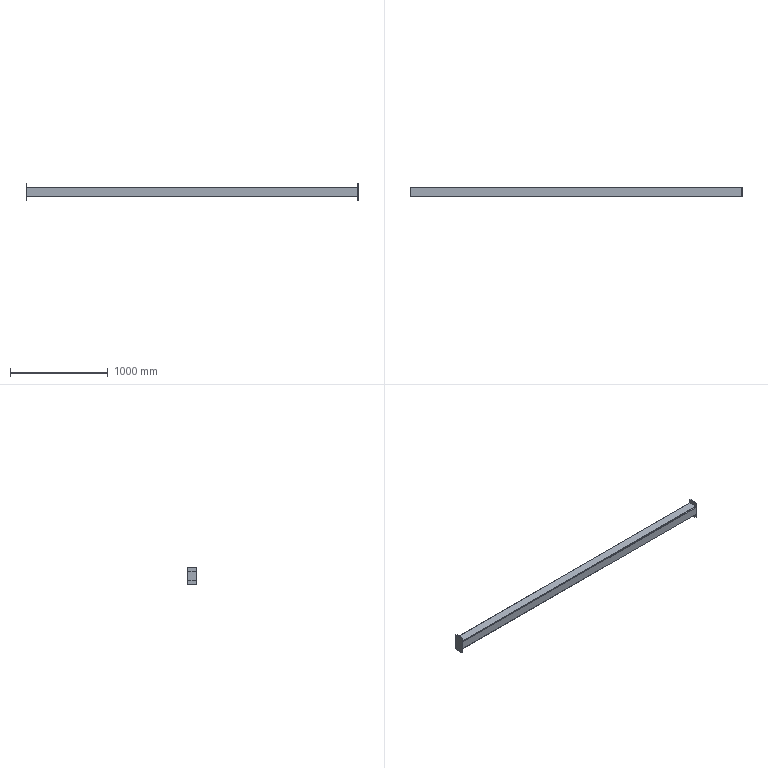Part | STEP file | Cross beam 2_Default<Machined> | 3 solids | 30 faces | box 3400 x 100 x 180 mm | volume 5412412 mm3 | plane 22 | cylinder 8 | commonest cylinder face diameters 8 x4 16 x4
STEP:
#1=CARTESIAN_POINT('',(-1690.,42.,-50.));
#2=VERTEX_POINT('',#1);
#3=CARTESIAN_POINT('',(-1690.,50.,-42.));
#4=VERTEX_POINT('',#3);
#5=CARTESIAN_POINT('',(-1690.,42.,-42.));
#6=DIRECTION('',(1.,0.,0.));
#7=DIRECTION('',(0.,0.,-1.));
#8=AXIS2_PLACEMENT_3D('',#5,#6,#7);
#9=CIRCLE('',#8,8.);
#10=EDGE_CURVE('',#2,#4,#9,.T.);
#11=ORIENTED_EDGE('',*,*,#10,.T.);
#12=CARTESIAN_POINT('',(1690.,50.,-42.));
#13=VERTEX_POINT('',#12);
#14=CARTESIAN_POINT('',(1690.,50.,-42.));
#15=DIRECTION('',(-1.,0.,0.));
#16=VECTOR('',#15,1000.);
#17=LINE('',#14,#16);
#18=EDGE_CURVE('',#13,#4,#17,.T.);
#19=ORIENTED_EDGE('',*,*,#18,.F.);
#20=CARTESIAN_POINT('',(1690.,42.,-50.));
#21=VERTEX_POINT('',#20);
#22=CARTESIAN_POINT('',(1690.,42.,-42.));
#23=DIRECTION('',(1.,0.,0.));
#24=DIRECTION('',(0.,0.,-1.));
#25=AXIS2_PLACEMENT_3D('',#22,#23,#24);
#26=CIRCLE('',#25,8.);
#27=EDGE_CURVE('',#21,#13,#26,.T.);
#28=ORIENTED_EDGE('',*,*,#27,.F.);
#29=CARTESIAN_POINT('',(1690.,42.,-50.));
#30=DIRECTION('',(-1.,0.,0.));
#31=VECTOR('',#30,1000.);
#32=LINE('',#29,#31);
#33=EDGE_CURVE('',#21,#2,#32,.T.);
#34=ORIENTED_EDGE('',*,*,#33,.T.);
#35=EDGE_LOOP('',(#11,#19,#28,#34));
#36=FACE_OUTER_BOUND('',#35,.T.);
#37=CARTESIAN_POINT('',(1690.,42.,-42.));
#38=DIRECTION('',(-1.,0.,0.));
#39=DIRECTION('',(0.,0.,1.));
#40=AXIS2_PLACEMENT_3D('',#37,#38,#39);
#41=CYLINDRICAL_SURFACE('',#40,8.);
#42=ADVANCED_FACE('',(#36),#41,.T.);
#43=CARTESIAN_POINT('',(-1690.,50.,42.));
#44=VERTEX_POINT('',#43);
#45=CARTESIAN_POINT('',(-1690.,50.,-42.));
#46=DIRECTION('',(0.,0.,1.));
#47=VECTOR('',#46,1000.);
#48=LINE('',#45,#47);
#49=EDGE_CURVE('',#4,#44,#48,.T.);
#50=ORIENTED_EDGE('',*,*,#49,.T.);
#51=CARTESIAN_POINT('',(1690.,50.,42.));
#52=VERTEX_POINT('',#51);
#53=CARTESIAN_POINT('',(1690.,50.,42.));
#54=DIRECTION('',(-1.,0.,0.));
#55=VECTOR('',#54,1000.);
#56=LINE('',#53,#55);
#57=EDGE_CURVE('',#52,#44,#56,.T.);
#58=ORIENTED_EDGE('',*,*,#57,.F.);
#59=CARTESIAN_POINT('',(1690.,50.,-42.));
#60=DIRECTION('',(0.,0.,1.));
#61=VECTOR('',#60,1000.);
#62=LINE('',#59,#61);
#63=EDGE_CURVE('',#13,#52,#62,.T.);
#64=ORIENTED_EDGE('',*,*,#63,.F.);
#65=ORIENTED_EDGE('',*,*,#18,.T.);
#66=EDGE_LOOP('',(#50,#58,#64,#65));
#67=FACE_OUTER_BOUND('',#66,.T.);
#68=CARTESIAN_POINT('',(1690.,50.,-42.));
#69=DIRECTION('',(0.,-1.,0.));
#70=DIRECTION('',(0.,0.,-1.));
#71=AXIS2_PLACEMENT_3D('',#68,#69,#70);
#72=PLANE('',#71);
#73=ADVANCED_FACE('',(#67),#72,.F.);
#74=CARTESIAN_POINT('',(-1690.,42.,50.));
#75=VERTEX_POINT('',#74);
#76=CARTESIAN_POINT('',(-1690.,42.,42.));
#77=DIRECTION('',(1.,0.,0.));
#78=DIRECTION('',(0.,0.,-1.));
#79=AXIS2_PLACEMENT_3D('',#76,#77,#78);
#80=CIRCLE('',#79,8.);
#81=EDGE_CURVE('',#44,#75,#80,.T.);
#82=ORIENTED_EDGE('',*,*,#81,.T.);
#83=CARTESIAN_POINT('',(1690.,42.,50.));
#84=VERTEX_POINT('',#83);
#85=CARTESIAN_POINT('',(1690.,42.,50.));
#86=DIRECTION('',(-1.,0.,0.));
#87=VECTOR('',#86,1000.);
#88=LINE('',#85,#87);
#89=EDGE_CURVE('',#84,#75,#88,.T.);
#90=ORIENTED_EDGE('',*,*,#89,.F.);
#91=CARTESIAN_POINT('',(1690.,42.,42.));
#92=DIRECTION('',(1.,0.,0.));
#93=DIRECTION('',(0.,0.,-1.));
#94=AXIS2_PLACEMENT_3D('',#91,#92,#93);
#95=CIRCLE('',#94,8.);
#96=EDGE_CURVE('',#52,#84,#95,.T.);
#97=ORIENTED_EDGE('',*,*,#96,.F.);
#98=ORIENTED_EDGE('',*,*,#57,.T.);
#99=EDGE_LOOP('',(#82,#90,#97,#98));
#100=FACE_OUTER_BOUND('',#99,.T.);
#101=CARTESIAN_POINT('',(1690.,42.,42.));
#102=DIRECTION('',(-1.,0.,0.));
#103=DIRECTION('',(0.,0.,1.));
#104=AXIS2_PLACEMENT_3D('',#101,#102,#103);
#105=CYLINDRICAL_SURFACE('',#104,8.);
#106=ADVANCED_FACE('',(#100),#105,.T.);
#107=CARTESIAN_POINT('',(-1690.,-42.,50.));
#108=VERTEX_POINT('',#107);
#109=CARTESIAN_POINT('',(-1690.,-42.,50.));
#110=DIRECTION('',(0.,-1.,0.));
#111=VECTOR('',#110,1000.);
#112=LINE('',#109,#111);
#113=EDGE_CURVE('',#75,#108,#112,.T.);
#114=ORIENTED_EDGE('',*,*,#113,.T.);
#115=CARTESIAN_POINT('',(1690.,-42.,50.));
#116=VERTEX_POINT('',#115);
#117=CARTESIAN_POINT('',(1690.,-42.,50.));
#118=DIRECTION('',(-1.,0.,0.));
#119=VECTOR('',#118,1000.);
#120=LINE('',#117,#119);
#121=EDGE_CURVE('',#116,#108,#120,.T.);
#122=ORIENTED_EDGE('',*,*,#121,.F.);
#123=CARTESIAN_POINT('',(1690.,-42.,50.));
#124=DIRECTION('',(0.,-1.,0.));
#125=VECTOR('',#124,1000.);
#126=LINE('',#123,#125);
#127=EDGE_CURVE('',#84,#116,#126,.T.);
#128=ORIENTED_EDGE('',*,*,#127,.F.);
#129=ORIENTED_EDGE('',*,*,#89,.T.);
#130=EDGE_LOOP('',(#114,#122,#128,#129));
#131=FACE_OUTER_BOUND('',#130,.T.);
#132=CARTESIAN_POINT('',(1690.,-42.,50.));
#133=DIRECTION('',(0.,0.,-1.));
#134=DIRECTION('',(-1.,0.,0.));
#135=AXIS2_PLACEMENT_3D('',#132,#133,#134);
#136=PLANE('',#135);
#137=ADVANCED_FACE('',(#131),#136,.F.);
#138=CARTESIAN_POINT('',(-1690.,-50.,42.));
#139=VERTEX_POINT('',#138);
#140=CARTESIAN_POINT('',(-1690.,-42.,42.));
#141=DIRECTION('',(1.,0.,0.));
#142=DIRECTION('',(0.,0.,-1.));
#143=AXIS2_PLACEMENT_3D('',#140,#141,#142);
#144=CIRCLE('',#143,8.);
#145=EDGE_CURVE('',#108,#139,#144,.T.);
#146=ORIENTED_EDGE('',*,*,#145,.T.);
#147=CARTESIAN_POINT('',(1690.,-50.,42.));
#148=VERTEX_POINT('',#147);
#149=CARTESIAN_POINT('',(1690.,-50.,42.));
#150=DIRECTION('',(-1.,0.,0.));
#151=VECTOR('',#150,1000.);
#152=LINE('',#149,#151);
#153=EDGE_CURVE('',#148,#139,#152,.T.);
#154=ORIENTED_EDGE('',*,*,#153,.F.);
#155=CARTESIAN_POINT('',(1690.,-42.,42.));
#156=DIRECTION('',(1.,0.,0.));
#157=DIRECTION('',(0.,0.,-1.));
#158=AXIS2_PLACEMENT_3D('',#155,#156,#157);
#159=CIRCLE('',#158,8.);
#160=EDGE_CURVE('',#116,#148,#159,.T.);
#161=ORIENTED_EDGE('',*,*,#160,.F.);
#162=ORIENTED_EDGE('',*,*,#121,.T.);
#163=EDGE_LOOP('',(#146,#154,#161,#162));
#164=FACE_OUTER_BOUND('',#163,.T.);
#165=CARTESIAN_POINT('',(1690.,-42.,42.));
#166=DIRECTION('',(-1.,0.,0.));
#167=DIRECTION('',(0.,0.,1.));
#168=AXIS2_PLACEMENT_3D('',#165,#166,#167);
#169=CYLINDRICAL_SURFACE('',#168,8.);
#170=ADVANCED_FACE('',(#164),#169,.T.);
#171=CARTESIAN_POINT('',(-1690.,-50.,-42.));
#172=VERTEX_POINT('',#171);
#173=CARTESIAN_POINT('',(-1690.,-50.,42.));
#174=DIRECTION('',(0.,0.,-1.));
#175=VECTOR('',#174,1000.);
#176=LINE('',#173,#175);
#177=EDGE_CURVE('',#139,#172,#176,.T.);
#178=ORIENTED_EDGE('',*,*,#177,.T.);
#179=CARTESIAN_POINT('',(1690.,-50.,-42.));
#180=VERTEX_POINT('',#179);
#181=CARTESIAN_POINT('',(1690.,-50.,-42.));
#182=DIRECTION('',(-1.,0.,0.));
#183=VECTOR('',#182,1000.);
#184=LINE('',#181,#183);
#185=EDGE_CURVE('',#180,#172,#184,.T.);
#186=ORIENTED_EDGE('',*,*,#185,.F.);
#187=CARTESIAN_POINT('',(1690.,-50.,42.));
#188=DIRECTION('',(0.,0.,-1.));
#189=VECTOR('',#188,1000.);
#190=LINE('',#187,#189);
#191=EDGE_CURVE('',#148,#180,#190,.T.);
#192=ORIENTED_EDGE('',*,*,#191,.F.);
#193=ORIENTED_EDGE('',*,*,#153,.T.);
#194=EDGE_LOOP('',(#178,#186,#192,#193));
#195=FACE_OUTER_BOUND('',#194,.T.);
#196=CARTESIAN_POINT('',(1690.,-50.,42.));
#197=DIRECTION('',(0.,1.,0.));
#198=DIRECTION('',(0.,0.,1.));
#199=AXIS2_PLACEMENT_3D('',#196,#197,#198);
#200=PLANE('',#199);
#201=ADVANCED_FACE('',(#195),#200,.F.);
#202=CARTESIAN_POINT('',(-1690.,-42.,-50.));
#203=VERTEX_POINT('',#202);
#204=CARTESIAN_POINT('',(-1690.,-42.,-42.));
#205=DIRECTION('',(1.,0.,0.));
#206=DIRECTION('',(0.,0.,-1.));
#207=AXIS2_PLACEMENT_3D('',#204,#205,#206);
#208=CIRCLE('',#207,8.);
#209=EDGE_CURVE('',#172,#203,#208,.T.);
#210=ORIENTED_EDGE('',*,*,#209,.T.);
#211=CARTESIAN_POINT('',(1690.,-42.,-50.));
#212=VERTEX_POINT('',#211);
#213=CARTESIAN_POINT('',(1690.,-42.,-50.));
#214=DIRECTION('',(-1.,0.,0.));
#215=VECTOR('',#214,1000.);
#216=LINE('',#213,#215);
#217=EDGE_CURVE('',#212,#203,#216,.T.);
#218=ORIENTED_EDGE('',*,*,#217,.F.);
#219=CARTESIAN_POINT('',(1690.,-42.,-42.));
#220=DIRECTION('',(1.,0.,0.));
#221=DIRECTION('',(0.,0.,-1.));
#222=AXIS2_PLACEMENT_3D('',#219,#220,#221);
#223=CIRCLE('',#222,8.);
#224=EDGE_CURVE('',#180,#212,#223,.T.);
#225=ORIENTED_EDGE('',*,*,#224,.F.);
#226=ORIENTED_EDGE('',*,*,#185,.T.);
#227=EDGE_LOOP('',(#210,#218,#225,#226));
#228=FACE_OUTER_BOUND('',#227,.T.);
#229=CARTESIAN_POINT('',(1690.,-42.,-42.));
#230=DIRECTION('',(-1.,0.,0.));
#231=DIRECTION('',(0.,0.,1.));
#232=AXIS2_PLACEMENT_3D('',#229,#230,#231);
#233=CYLINDRICAL_SURFACE('',#232,8.);
#234=ADVANCED_FACE('',(#228),#233,.T.);
#235=CARTESIAN_POINT('',(-1690.,46.,42.));
#236=VERTEX_POINT('',#235);
#237=CARTESIAN_POINT('',(-1690.,42.,46.));
#238=VERTEX_POINT('',#237);
#239=CARTESIAN_POINT('',(-1690.,42.,42.));
#240=DIRECTION('',(1.,0.,0.));
#241=DIRECTION('',(0.,0.,-1.));
#242=AXIS2_PLACEMENT_3D('',#239,#240,#241);
#243=CIRCLE('',#242,4.);
#244=EDGE_CURVE('',#236,#238,#243,.T.);
#245=ORIENTED_EDGE('',*,*,#244,.F.);
#246=CARTESIAN_POINT('',(1690.,46.,42.));
#247=VERTEX_POINT('',#246);
#248=CARTESIAN_POINT('',(1690.,46.,42.));
#249=DIRECTION('',(-1.,0.,0.));
#250=VECTOR('',#249,1000.);
#251=LINE('',#248,#250);
#252=EDGE_CURVE('',#247,#236,#251,.T.);
#253=ORIENTED_EDGE('',*,*,#252,.F.);
#254=CARTESIAN_POINT('',(1690.,42.,46.));
#255=VERTEX_POINT('',#254);
#256=CARTESIAN_POINT('',(1690.,42.,42.));
#257=DIRECTION('',(1.,0.,0.));
#258=DIRECTION('',(0.,0.,-1.));
#259=AXIS2_PLACEMENT_3D('',#256,#257,#258);
#260=CIRCLE('',#259,4.);
#261=EDGE_CURVE('',#247,#255,#260,.T.);
#262=ORIENTED_EDGE('',*,*,#261,.T.);
#263=CARTESIAN_POINT('',(1690.,42.,46.));
#264=DIRECTION('',(-1.,0.,0.));
#265=VECTOR('',#264,1000.);
#266=LINE('',#263,#265);
#267=EDGE_CURVE('',#255,#238,#266,.T.);
#268=ORIENTED_EDGE('',*,*,#267,.T.);
#269=EDGE_LOOP('',(#245,#253,#262,#268));
#270=FACE_OUTER_BOUND('',#269,.T.);
#271=CARTESIAN_POINT('',(1690.,42.,42.));
#272=DIRECTION('',(-1.,0.,0.));
#273=DIRECTION('',(0.,0.,1.));
#274=AXIS2_PLACEMENT_3D('',#271,#272,#273);
#275=CYLINDRICAL_SURFACE('',#274,4.);
#276=ADVANCED_FACE('',(#270),#275,.F.);
#277=CARTESIAN_POINT('',(-1690.,46.,-42.));
#278=VERTEX_POINT('',#277);
#279=CARTESIAN_POINT('',(-1690.,46.,-42.));
#280=DIRECTION('',(0.,0.,1.));
#281=VECTOR('',#280,1000.);
#282=LINE('',#279,#281);
#283=EDGE_CURVE('',#278,#236,#282,.T.);
#284=ORIENTED_EDGE('',*,*,#283,.F.);
#285=CARTESIAN_POINT('',(1690.,46.,-42.));
#286=VERTEX_POINT('',#285);
#287=CARTESIAN_POINT('',(1690.,46.,-42.));
#288=DIRECTION('',(-1.,0.,0.));
#289=VECTOR('',#288,1000.);
#290=LINE('',#287,#289);
#291=EDGE_CURVE('',#286,#278,#290,.T.);
#292=ORIENTED_EDGE('',*,*,#291,.F.);
#293=CARTESIAN_POINT('',(1690.,46.,-42.));
#294=DIRECTION('',(0.,0.,1.));
#295=VECTOR('',#294,1000.);
#296=LINE('',#293,#295);
#297=EDGE_CURVE('',#286,#247,#296,.T.);
#298=ORIENTED_EDGE('',*,*,#297,.T.);
#299=ORIENTED_EDGE('',*,*,#252,.T.);
#300=EDGE_LOOP('',(#284,#292,#298,#299));
#301=FACE_OUTER_BOUND('',#300,.T.);
#302=CARTESIAN_POINT('',(1690.,46.,-42.));
#303=DIRECTION('',(0.,-1.,0.));
#304=DIRECTION('',(0.,0.,-1.));
#305=AXIS2_PLACEMENT_3D('',#302,#303,#304);
#306=PLANE('',#305);
#307=ADVANCED_FACE('',(#301),#306,.T.);
#308=CARTESIAN_POINT('',(-1690.,42.,-46.));
#309=VERTEX_POINT('',#308);
#310=CARTESIAN_POINT('',(-1690.,42.,-42.));
#311=DIRECTION('',(1.,0.,0.));
#312=DIRECTION('',(0.,0.,-1.));
#313=AXIS2_PLACEMENT_3D('',#310,#311,#312);
#314=CIRCLE('',#313,4.);
#315=EDGE_CURVE('',#309,#278,#314,.T.);
#316=ORIENTED_EDGE('',*,*,#315,.F.);
#317=CARTESIAN_POINT('',(1690.,42.,-46.));
#318=VERTEX_POINT('',#317);
#319=CARTESIAN_POINT('',(1690.,42.,-46.));
#320=DIRECTION('',(-1.,0.,0.));
#321=VECTOR('',#320,1000.);
#322=LINE('',#319,#321);
#323=EDGE_CURVE('',#318,#309,#322,.T.);
#324=ORIENTED_EDGE('',*,*,#323,.F.);
#325=CARTESIAN_POINT('',(1690.,42.,-42.));
#326=DIRECTION('',(1.,0.,0.));
#327=DIRECTION('',(0.,0.,-1.));
#328=AXIS2_PLACEMENT_3D('',#325,#326,#327);
#329=CIRCLE('',#328,4.);
#330=EDGE_CURVE('',#318,#286,#329,.T.);
#331=ORIENTED_EDGE('',*,*,#330,.T.);
#332=ORIENTED_EDGE('',*,*,#291,.T.);
#333=EDGE_LOOP('',(#316,#324,#331,#332));
#334=FACE_OUTER_BOUND('',#333,.T.);
#335=CARTESIAN_POINT('',(1690.,42.,-42.));
#336=DIRECTION('',(-1.,0.,0.));
#337=DIRECTION('',(0.,0.,1.));
#338=AXIS2_PLACEMENT_3D('',#335,#336,#337);
#339=CYLINDRICAL_SURFACE('',#338,4.);
#340=ADVANCED_FACE('',(#334),#339,.F.);
#341=CARTESIAN_POINT('',(-1690.,-42.,-46.));
#342=VERTEX_POINT('',#341);
#343=CARTESIAN_POINT('',(-1690.,42.,-46.));
#344=DIRECTION('',(0.,1.,0.));
#345=VECTOR('',#344,1000.);
#346=LINE('',#343,#345);
#347=EDGE_CURVE('',#342,#309,#346,.T.);
#348=ORIENTED_EDGE('',*,*,#347,.F.);
#349=CARTESIAN_POINT('',(1690.,-42.,-46.));
#350=VERTEX_POINT('',#349);
#351=CARTESIAN_POINT('',(1690.,-42.,-46.));
#352=DIRECTION('',(-1.,0.,0.));
#353=VECTOR('',#352,1000.);
#354=LINE('',#351,#353);
#355=EDGE_CURVE('',#350,#342,#354,.T.);
#356=ORIENTED_EDGE('',*,*,#355,.F.);
#357=CARTESIAN_POINT('',(1690.,42.,-46.));
#358=DIRECTION('',(0.,1.,0.));
#359=VECTOR('',#358,1000.);
#360=LINE('',#357,#359);
#361=EDGE_CURVE('',#350,#318,#360,.T.);
#362=ORIENTED_EDGE('',*,*,#361,.T.);
#363=ORIENTED_EDGE('',*,*,#323,.T.);
#364=EDGE_LOOP('',(#348,#356,#362,#363));
#365=FACE_OUTER_BOUND('',#364,.T.);
#366=CARTESIAN_POINT('',(1690.,42.,-46.));
#367=DIRECTION('',(0.,0.,1.));
#368=DIRECTION('',(1.,0.,0.));
#369=AXIS2_PLACEMENT_3D('',#366,#367,#368);
#370=PLANE('',#369);
#371=ADVANCED_FACE('',(#365),#370,.T.);
#372=CARTESIAN_POINT('',(-1690.,-46.,-42.));
#373=VERTEX_POINT('',#372);
#374=CARTESIAN_POINT('',(-1690.,-42.,-42.));
#375=DIRECTION('',(1.,0.,0.));
#376=DIRECTION('',(0.,0.,-1.));
#377=AXIS2_PLACEMENT_3D('',#374,#375,#376);
#378=CIRCLE('',#377,4.);
#379=EDGE_CURVE('',#373,#342,#378,.T.);
#380=ORIENTED_EDGE('',*,*,#379,.F.);
#381=CARTESIAN_POINT('',(1690.,-46.,-42.));
#382=VERTEX_POINT('',#381);
#383=CARTESIAN_POINT('',(1690.,-46.,-42.));
#384=DIRECTION('',(-1.,0.,0.));
#385=VECTOR('',#384,1000.);
#386=LINE('',#383,#385);
#387=EDGE_CURVE('',#382,#373,#386,.T.);
#388=ORIENTED_EDGE('',*,*,#387,.F.);
#389=CARTESIAN_POINT('',(1690.,-42.,-42.));
#390=DIRECTION('',(1.,0.,0.));
#391=DIRECTION('',(0.,0.,-1.));
#392=AXIS2_PLACEMENT_3D('',#389,#390,#391);
#393=CIRCLE('',#392,4.);
#394=EDGE_CURVE('',#382,#350,#393,.T.);
#395=ORIENTED_EDGE('',*,*,#394,.T.);
#396=ORIENTED_EDGE('',*,*,#355,.T.);
#397=EDGE_LOOP('',(#380,#388,#395,#396));
#398=FACE_OUTER_BOUND('',#397,.T.);
#399=CARTESIAN_POINT('',(1690.,-42.,-42.));
#400=DIRECTION('',(-1.,0.,0.));
#401=DIRECTION('',(0.,0.,1.));
#402=AXIS2_PLACEMENT_3D('',#399,#400,#401);
#403=CYLINDRICAL_SURFACE('',#402,4.);
#404=ADVANCED_FACE('',(#398),#403,.F.);
#405=CARTESIAN_POINT('',(-1690.,-46.,42.));
#406=VERTEX_POINT('',#405);
#407=CARTESIAN_POINT('',(-1690.,-46.,42.));
#408=DIRECTION('',(0.,0.,-1.));
#409=VECTOR('',#408,1000.);
#410=LINE('',#407,#409);
#411=EDGE_CURVE('',#406,#373,#410,.T.);
#412=ORIENTED_EDGE('',*,*,#411,.F.);
#413=CARTESIAN_POINT('',(1690.,-46.,42.));
#414=VERTEX_POINT('',#413);
#415=CARTESIAN_POINT('',(1690.,-46.,42.));
#416=DIRECTION('',(-1.,0.,0.));
#417=VECTOR('',#416,1000.);
#418=LINE('',#415,#417);
#419=EDGE_CURVE('',#414,#406,#418,.T.);
#420=ORIENTED_EDGE('',*,*,#419,.F.);
#421=CARTESIAN_POINT('',(1690.,-46.,42.));
#422=DIRECTION('',(0.,0.,-1.));
#423=VECTOR('',#422,1000.);
#424=LINE('',#421,#423);
#425=EDGE_CURVE('',#414,#382,#424,.T.);
#426=ORIENTED_EDGE('',*,*,#425,.T.);
#427=ORIENTED_EDGE('',*,*,#387,.T.);
#428=EDGE_LOOP('',(#412,#420,#426,#427));
#429=FACE_OUTER_BOUND('',#428,.T.);
#430=CARTESIAN_POINT('',(1690.,-46.,42.));
#431=DIRECTION('',(0.,1.,0.));
#432=DIRECTION('',(0.,0.,1.));
#433=AXIS2_PLACEMENT_3D('',#430,#431,#432);
#434=PLANE('',#433);
#435=ADVANCED_FACE('',(#429),#434,.T.);
#436=CARTESIAN_POINT('',(-1690.,-42.,46.));
#437=VERTEX_POINT('',#436);
#438=CARTESIAN_POINT('',(-1690.,-42.,42.));
#439=DIRECTION('',(1.,0.,0.));
#440=DIRECTION('',(0.,0.,-1.));
#441=AXIS2_PLACEMENT_3D('',#438,#439,#440);
#442=CIRCLE('',#441,4.);
#443=EDGE_CURVE('',#437,#406,#442,.T.);
#444=ORIENTED_EDGE('',*,*,#443,.F.);
#445=CARTESIAN_POINT('',(1690.,-42.,46.));
#446=VERTEX_POINT('',#445);
#447=CARTESIAN_POINT('',(1690.,-42.,46.));
#448=DIRECTION('',(-1.,0.,0.));
#449=VECTOR('',#448,1000.);
#450=LINE('',#447,#449);
#451=EDGE_CURVE('',#446,#437,#450,.T.);
#452=ORIENTED_EDGE('',*,*,#451,.F.);
#453=CARTESIAN_POINT('',(1690.,-42.,42.));
#454=DIRECTION('',(1.,0.,0.));
#455=DIRECTION('',(0.,0.,-1.));
#456=AXIS2_PLACEMENT_3D('',#453,#454,#455);
#457=CIRCLE('',#456,4.);
#458=EDGE_CURVE('',#446,#414,#457,.T.);
#459=ORIENTED_EDGE('',*,*,#458,.T.);
#460=ORIENTED_EDGE('',*,*,#419,.T.);
#461=EDGE_LOOP('',(#444,#452,#459,#460));
#462=FACE_OUTER_BOUND('',#461,.T.);
#463=CARTESIAN_POINT('',(1690.,-42.,42.));
#464=DIRECTION('',(-1.,0.,0.));
#465=DIRECTION('',(0.,0.,1.));
#466=AXIS2_PLACEMENT_3D('',#463,#464,#465);
#467=CYLINDRICAL_SURFACE('',#466,4.);
#468=ADVANCED_FACE('',(#462),#467,.F.);
#469=CARTESIAN_POINT('',(-1690.,-42.,46.));
#470=DIRECTION('',(0.,-1.,0.));
#471=VECTOR('',#470,1000.);
#472=LINE('',#469,#471);
#473=EDGE_CURVE('',#238,#437,#472,.T.);
#474=ORIENTED_EDGE('',*,*,#473,.F.);
#475=ORIENTED_EDGE('',*,*,#267,.F.);
#476=CARTESIAN_POINT('',(1690.,-42.,46.));
#477=DIRECTION('',(0.,-1.,0.));
#478=VECTOR('',#477,1000.);
#479=LINE('',#476,#478);
#480=EDGE_CURVE('',#255,#446,#479,.T.);
#481=ORIENTED_EDGE('',*,*,#480,.T.);
#482=ORIENTED_EDGE('',*,*,#451,.T.);
#483=EDGE_LOOP('',(#474,#475,#481,#482));
#484=FACE_OUTER_BOUND('',#483,.T.);
#485=CARTESIAN_POINT('',(1690.,-42.,46.));
#486=DIRECTION('',(0.,0.,-1.));
#487=DIRECTION('',(-1.,0.,0.));
#488=AXIS2_PLACEMENT_3D('',#485,#486,#487);
#489=PLANE('',#488);
#490=ADVANCED_FACE('',(#484),#489,.T.);
#491=CARTESIAN_POINT('',(-1690.,42.,-50.));
#492=DIRECTION('',(0.,1.,0.));
#493=VECTOR('',#492,1000.);
#494=LINE('',#491,#493);
#495=EDGE_CURVE('',#203,#2,#494,.T.);
#496=ORIENTED_EDGE('',*,*,#495,.T.);
#497=ORIENTED_EDGE('',*,*,#33,.F.);
#498=CARTESIAN_POINT('',(1690.,42.,-50.));
#499=DIRECTION('',(0.,1.,0.));
#500=VECTOR('',#499,1000.);
#501=LINE('',#498,#500);
#502=EDGE_CURVE('',#212,#21,#501,.T.);
#503=ORIENTED_EDGE('',*,*,#502,.F.);
#504=ORIENTED_EDGE('',*,*,#217,.T.);
#505=EDGE_LOOP('',(#496,#497,#503,#504));
#506=FACE_OUTER_BOUND('',#505,.T.);
#507=CARTESIAN_POINT('',(1690.,42.,-50.));
#508=DIRECTION('',(0.,0.,1.));
#509=DIRECTION('',(1.,0.,0.));
#510=AXIS2_PLACEMENT_3D('',#507,#508,#509);
#511=PLANE('',#510);
#512=ADVANCED_FACE('',(#506),#511,.F.);
#513=ORIENTED_EDGE('',*,*,#261,.F.);
#514=ORIENTED_EDGE('',*,*,#297,.F.);
#515=ORIENTED_EDGE('',*,*,#330,.F.);
#516=ORIENTED_EDGE('',*,*,#361,.F.);
#517=ORIENTED_EDGE('',*,*,#394,.F.);
#518=ORIENTED_EDGE('',*,*,#425,.F.);
#519=ORIENTED_EDGE('',*,*,#458,.F.);
#520=ORIENTED_EDGE('',*,*,#480,.F.);
#521=EDGE_LOOP('',(#513,#514,#515,#516,#517,#518,#519,#520));
#522=FACE_BOUND('',#521,.T.);
#523=ORIENTED_EDGE('',*,*,#27,.T.);
#524=ORIENTED_EDGE('',*,*,#63,.T.);
#525=ORIENTED_EDGE('',*,*,#96,.T.);
#526=ORIENTED_EDGE('',*,*,#127,.T.);
#527=ORIENTED_EDGE('',*,*,#160,.T.);
#528=ORIENTED_EDGE('',*,*,#191,.T.);
#529=ORIENTED_EDGE('',*,*,#224,.T.);
#530=ORIENTED_EDGE('',*,*,#502,.T.);
#531=EDGE_LOOP('',(#523,#524,#525,#526,#527,#528,#529,#530));
#532=FACE_OUTER_BOUND('',#531,.T.);
#533=CARTESIAN_POINT('',(1690.,42.,-42.));
#534=DIRECTION('',(1.,0.,0.));
#535=DIRECTION('',(0.,0.,-1.));
#536=AXIS2_PLACEMENT_3D('',#533,#534,#535);
#537=PLANE('',#536);
#538=ADVANCED_FACE('',(#522,#532),#537,.T.);
#539=ORIENTED_EDGE('',*,*,#244,.T.);
#540=ORIENTED_EDGE('',*,*,#473,.T.);
#541=ORIENTED_EDGE('',*,*,#443,.T.);
#542=ORIENTED_EDGE('',*,*,#411,.T.);
#543=ORIENTED_EDGE('',*,*,#379,.T.);
#544=ORIENTED_EDGE('',*,*,#347,.T.);
#545=ORIENTED_EDGE('',*,*,#315,.T.);
#546=ORIENTED_EDGE('',*,*,#283,.T.);
#547=EDGE_LOOP('',(#539,#540,#541,#542,#543,#544,#545,#546));
#548=FACE_BOUND('',#547,.T.);
#549=ORIENTED_EDGE('',*,*,#10,.F.);
#550=ORIENTED_EDGE('',*,*,#495,.F.);
#551=ORIENTED_EDGE('',*,*,#209,.F.);
#552=ORIENTED_EDGE('',*,*,#177,.F.);
#553=ORIENTED_EDGE('',*,*,#145,.F.);
#554=ORIENTED_EDGE('',*,*,#113,.F.);
#555=ORIENTED_EDGE('',*,*,#81,.F.);
#556=ORIENTED_EDGE('',*,*,#49,.F.);
#557=EDGE_LOOP('',(#549,#550,#551,#552,#553,#554,#555,#556));
#558=FACE_OUTER_BOUND('',#557,.T.);
#559=CARTESIAN_POINT('',(-1690.,42.,-42.));
#560=DIRECTION('',(1.,0.,0.));
#561=DIRECTION('',(0.,0.,-1.));
#562=AXIS2_PLACEMENT_3D('',#559,#560,#561);
#563=PLANE('',#562);
#564=ADVANCED_FACE('',(#548,#558),#563,.F.);
#565=CLOSED_SHELL('',(#42,#73,#106,#137,#170,#201,#234,#276,#307,#340,#371,#404,#435,#468,#490,#512,#538,#564));
#566=MANIFOLD_SOLID_BREP('',#565);
#567=CARTESIAN_POINT('',(-1690.,-50.,90.));
#568=VERTEX_POINT('',#567);
#569=CARTESIAN_POINT('',(-1690.,50.,90.));
#570=VERTEX_POINT('',#569);
#571=CARTESIAN_POINT('',(-1690.,-50.,90.));
#572=DIRECTION('',(0.,1.,0.));
#573=VECTOR('',#572,1000.);
#574=LINE('',#571,#573);
#575=EDGE_CURVE('',#568,#570,#574,.T.);
#576=ORIENTED_EDGE('',*,*,#575,.T.);
#577=CARTESIAN_POINT('',(-1700.,50.,90.));
#578=VERTEX_POINT('',#577);
#579=CARTESIAN_POINT('',(-1700.,50.,90.));
#580=DIRECTION('',(1.,0.,0.));
#581=VECTOR('',#580,1000.);
#582=LINE('',#579,#581);
#583=EDGE_CURVE('',#578,#570,#582,.T.);
#584=ORIENTED_EDGE('',*,*,#583,.F.);
#585=CARTESIAN_POINT('',(-1700.,-50.,90.));
#586=VERTEX_POINT('',#585);
#587=CARTESIAN_POINT('',(-1700.,-50.,90.));
#588=DIRECTION('',(0.,1.,0.));
#589=VECTOR('',#588,1000.);
#590=LINE('',#587,#589);
#591=EDGE_CURVE('',#586,#578,#590,.T.);
#592=ORIENTED_EDGE('',*,*,#591,.F.);
#593=CARTESIAN_POINT('',(-1700.,-50.,90.));
#594=DIRECTION('',(1.,0.,0.));
#595=VECTOR('',#594,1000.);
#596=LINE('',#593,#595);
#597=EDGE_CURVE('',#586,#568,#596,.T.);
#598=ORIENTED_EDGE('',*,*,#597,.T.);
#599=EDGE_LOOP('',(#576,#584,#592,#598));
#600=FACE_OUTER_BOUND('',#599,.T.);
#601=CARTESIAN_POINT('',(-1700.,-50.,90.));
#602=DIRECTION('',(0.,0.,-1.));
#603=DIRECTION('',(-1.,0.,0.));
#604=AXIS2_PLACEMENT_3D('',#601,#602,#603);
#605=PLANE('',#604);
#606=ADVANCED_FACE('',(#600),#605,.F.);
#607=CARTESIAN_POINT('',(-1690.,50.,-90.));
#608=VERTEX_POINT('',#607);
#609=CARTESIAN_POINT('',(-1690.,50.,-90.));
#610=DIRECTION('',(0.,0.,-1.));
#611=VECTOR('',#610,1000.);
#612=LINE('',#609,#611);
#613=EDGE_CURVE('',#570,#608,#612,.T.);
#614=ORIENTED_EDGE('',*,*,#613,.T.);
#615=CARTESIAN_POINT('',(-1700.,50.,-90.));
#616=VERTEX_POINT('',#615);
#617=CARTESIAN_POINT('',(-1700.,50.,-90.));
#618=DIRECTION('',(1.,0.,0.));
#619=VECTOR('',#618,1000.);
#620=LINE('',#617,#619);
#621=EDGE_CURVE('',#616,#608,#620,.T.);
#622=ORIENTED_EDGE('',*,*,#621,.F.);
#623=CARTESIAN_POINT('',(-1700.,50.,-90.));
#624=DIRECTION('',(0.,0.,-1.));
#625=VECTOR('',#624,1000.);
#626=LINE('',#623,#625);
#627=EDGE_CURVE('',#578,#616,#626,.T.);
#628=ORIENTED_EDGE('',*,*,#627,.F.);
#629=ORIENTED_EDGE('',*,*,#583,.T.);
#630=EDGE_LOOP('',(#614,#622,#628,#629));
#631=FACE_OUTER_BOUND('',#630,.T.);
#632=CARTESIAN_POINT('',(-1700.,50.,-90.));
#633=DIRECTION('',(0.,-1.,0.));
#634=DIRECTION('',(0.,0.,-1.));
#635=AXIS2_PLACEMENT_3D('',#632,#633,#634);
#636=PLANE('',#635);
#637=ADVANCED_FACE('',(#631),#636,.F.);
#638=CARTESIAN_POINT('',(-1690.,-50.,-90.));
#639=VERTEX_POINT('',#638);
#640=CARTESIAN_POINT('',(-1690.,-50.,-90.));
#641=DIRECTION('',(0.,-1.,0.));
#642=VECTOR('',#641,1000.);
#643=LINE('',#640,#642);
#644=EDGE_CURVE('',#608,#639,#643,.T.);
#645=ORIENTED_EDGE('',*,*,#644,.T.);
#646=CARTESIAN_POINT('',(-1700.,-50.,-90.));
#647=VERTEX_POINT('',#646);
#648=CARTESIAN_POINT('',(-1700.,-50.,-90.));
#649=DIRECTION('',(1.,0.,0.));
#650=VECTOR('',#649,1000.);
#651=LINE('',#648,#650);
#652=EDGE_CURVE('',#647,#639,#651,.T.);
#653=ORIENTED_EDGE('',*,*,#652,.F.);
#654=CARTESIAN_POINT('',(-1700.,-50.,-90.));
#655=DIRECTION('',(0.,-1.,0.));
#656=VECTOR('',#655,1000.);
#657=LINE('',#654,#656);
#658=EDGE_CURVE('',#616,#647,#657,.T.);
#659=ORIENTED_EDGE('',*,*,#658,.F.);
#660=ORIENTED_EDGE('',*,*,#621,.T.);
#661=EDGE_LOOP('',(#645,#653,#659,#660));
#662=FACE_OUTER_BOUND('',#661,.T.);
#663=CARTESIAN_POINT('',(-1700.,-50.,-90.));
#664=DIRECTION('',(0.,0.,1.));
#665=DIRECTION('',(1.,0.,0.));
#666=AXIS2_PLACEMENT_3D('',#663,#664,#665);
#667=PLANE('',#666);
#668=ADVANCED_FACE('',(#662),#667,.F.);
#669=CARTESIAN_POINT('',(-1690.,-50.,-90.));
#670=DIRECTION('',(0.,0.,1.));
#671=VECTOR('',#670,1000.);
#672=LINE('',#669,#671);
#673=EDGE_CURVE('',#639,#568,#672,.T.);
#674=ORIENTED_EDGE('',*,*,#673,.T.);
#675=ORIENTED_EDGE('',*,*,#597,.F.);
#676=CARTESIAN_POINT('',(-1700.,-50.,-90.));
#677=DIRECTION('',(0.,0.,1.));
#678=VECTOR('',#677,1000.);
#679=LINE('',#676,#678);
#680=EDGE_CURVE('',#647,#586,#679,.T.);
#681=ORIENTED_EDGE('',*,*,#680,.F.);
#682=ORIENTED_EDGE('',*,*,#652,.T.);
#683=EDGE_LOOP('',(#674,#675,#681,#682));
#684=FACE_OUTER_BOUND('',#683,.T.);
#685=CARTESIAN_POINT('',(-1700.,-50.,-90.));
#686=DIRECTION('',(0.,1.,0.));
#687=DIRECTION('',(0.,0.,1.));
#688=AXIS2_PLACEMENT_3D('',#685,#686,#687);
#689=PLANE('',#688);
#690=ADVANCED_FACE('',(#684),#689,.F.);
#691=ORIENTED_EDGE('',*,*,#591,.T.);
#692=ORIENTED_EDGE('',*,*,#627,.T.);
#693=ORIENTED_EDGE('',*,*,#658,.T.);
#694=ORIENTED_EDGE('',*,*,#680,.T.);
#695=EDGE_LOOP('',(#691,#692,#693,#694));
#696=FACE_OUTER_BOUND('',#695,.T.);
#697=CARTESIAN_POINT('',(-1700.,0.,0.));
#698=DIRECTION('',(1.,0.,0.));
#699=DIRECTION('',(0.,0.,-1.));
#700=AXIS2_PLACEMENT_3D('',#697,#698,#699);
#701=PLANE('',#700);
#702=ADVANCED_FACE('',(#696),#701,.F.);
#703=ORIENTED_EDGE('',*,*,#575,.F.);
#704=ORIENTED_EDGE('',*,*,#673,.F.);
#705=ORIENTED_EDGE('',*,*,#644,.F.);
#706=ORIENTED_EDGE('',*,*,#613,.F.);
#707=EDGE_LOOP('',(#703,#704,#705,#706));
#708=FACE_OUTER_BOUND('',#707,.T.);
#709=CARTESIAN_POINT('',(-1690.,0.,0.));
#710=DIRECTION('',(1.,0.,0.));
#711=DIRECTION('',(0.,0.,-1.));
#712=AXIS2_PLACEMENT_3D('',#709,#710,#711);
#713=PLANE('',#712);
#714=ADVANCED_FACE('',(#708),#713,.T.);
#715=CLOSED_SHELL('',(#606,#637,#668,#690,#702,#714));
#716=MANIFOLD_SOLID_BREP('',#715);
#717=CARTESIAN_POINT('',(1690.,-50.,90.));
#718=VERTEX_POINT('',#717);
#719=CARTESIAN_POINT('',(1690.,50.,90.));
#720=VERTEX_POINT('',#719);
#721=CARTESIAN_POINT('',(1690.,-50.,90.));
#722=DIRECTION('',(0.,1.,0.));
#723=VECTOR('',#722,1000.);
#724=LINE('',#721,#723);
#725=EDGE_CURVE('',#718,#720,#724,.T.);
#726=ORIENTED_EDGE('',*,*,#725,.F.);
#727=CARTESIAN_POINT('',(1700.,-50.,90.));
#728=VERTEX_POINT('',#727);
#729=CARTESIAN_POINT('',(1700.,-50.,90.));
#730=DIRECTION('',(-1.,0.,0.));
#731=VECTOR('',#730,1000.);
#732=LINE('',#729,#731);
#733=EDGE_CURVE('',#728,#718,#732,.T.);
#734=ORIENTED_EDGE('',*,*,#733,.F.);
#735=CARTESIAN_POINT('',(1700.,50.,90.));
#736=VERTEX_POINT('',#735);
#737=CARTESIAN_POINT('',(1700.,-50.,90.));
#738=DIRECTION('',(0.,1.,0.));
#739=VECTOR('',#738,1000.);
#740=LINE('',#737,#739);
#741=EDGE_CURVE('',#728,#736,#740,.T.);
#742=ORIENTED_EDGE('',*,*,#741,.T.);
#743=CARTESIAN_POINT('',(1700.,50.,90.));
#744=DIRECTION('',(-1.,0.,0.));
#745=VECTOR('',#744,1000.);
#746=LINE('',#743,#745);
#747=EDGE_CURVE('',#736,#720,#746,.T.);
#748=ORIENTED_EDGE('',*,*,#747,.T.);
#749=EDGE_LOOP('',(#726,#734,#742,#748));
#750=FACE_OUTER_BOUND('',#749,.T.);
#751=CARTESIAN_POINT('',(1700.,-50.,90.));
#752=DIRECTION('',(0.,0.,-1.));
#753=DIRECTION('',(1.,0.,0.));
#754=AXIS2_PLACEMENT_3D('',#751,#752,#753);
#755=PLANE('',#754);
#756=ADVANCED_FACE('',(#750),#755,.F.);
#757=CARTESIAN_POINT('',(1690.,50.,-90.));
#758=VERTEX_POINT('',#757);
#759=CARTESIAN_POINT('',(1690.,50.,-90.));
#760=DIRECTION('',(0.,0.,-1.));
#761=VECTOR('',#760,1000.);
#762=LINE('',#759,#761);
#763=EDGE_CURVE('',#720,#758,#762,.T.);
#764=ORIENTED_EDGE('',*,*,#763,.F.);
#765=ORIENTED_EDGE('',*,*,#747,.F.);
#766=CARTESIAN_POINT('',(1700.,50.,-90.));
#767=VERTEX_POINT('',#766);
#768=CARTESIAN_POINT('',(1700.,50.,-90.));
#769=DIRECTION('',(0.,0.,-1.));
#770=VECTOR('',#769,1000.);
#771=LINE('',#768,#770);
#772=EDGE_CURVE('',#736,#767,#771,.T.);
#773=ORIENTED_EDGE('',*,*,#772,.T.);
#774=CARTESIAN_POINT('',(1700.,50.,-90.));
#775=DIRECTION('',(-1.,0.,0.));
#776=VECTOR('',#775,1000.);
#777=LINE('',#774,#776);
#778=EDGE_CURVE('',#767,#758,#777,.T.);
#779=ORIENTED_EDGE('',*,*,#778,.T.);
#780=EDGE_LOOP('',(#764,#765,#773,#779));
#781=FACE_OUTER_BOUND('',#780,.T.);
#782=CARTESIAN_POINT('',(1700.,50.,-90.));
#783=DIRECTION('',(0.,-1.,0.));
#784=DIRECTION('',(0.,0.,-1.));
#785=AXIS2_PLACEMENT_3D('',#782,#783,#784);
#786=PLANE('',#785);
#787=ADVANCED_FACE('',(#781),#786,.F.);
#788=CARTESIAN_POINT('',(1690.,-50.,-90.));
#789=VERTEX_POINT('',#788);
#790=CARTESIAN_POINT('',(1690.,-50.,-90.));
#791=DIRECTION('',(0.,-1.,0.));
#792=VECTOR('',#791,1000.);
#793=LINE('',#790,#792);
#794=EDGE_CURVE('',#758,#789,#793,.T.);
#795=ORIENTED_EDGE('',*,*,#794,.F.);
#796=ORIENTED_EDGE('',*,*,#778,.F.);
#797=CARTESIAN_POINT('',(1700.,-50.,-90.));
#798=VERTEX_POINT('',#797);
#799=CARTESIAN_POINT('',(1700.,-50.,-90.));
#800=DIRECTION('',(0.,-1.,0.));
#801=VECTOR('',#800,1000.);
#802=LINE('',#799,#801);
#803=EDGE_CURVE('',#767,#798,#802,.T.);
#804=ORIENTED_EDGE('',*,*,#803,.T.);
#805=CARTESIAN_POINT('',(1700.,-50.,-90.));
#806=DIRECTION('',(-1.,0.,0.));
#807=VECTOR('',#806,1000.);
#808=LINE('',#805,#807);
#809=EDGE_CURVE('',#798,#789,#808,.T.);
#810=ORIENTED_EDGE('',*,*,#809,.T.);
#811=EDGE_LOOP('',(#795,#796,#804,#810));
#812=FACE_OUTER_BOUND('',#811,.T.);
#813=CARTESIAN_POINT('',(1700.,-50.,-90.));
#814=DIRECTION('',(0.,0.,1.));
#815=DIRECTION('',(-1.,0.,0.));
#816=AXIS2_PLACEMENT_3D('',#813,#814,#815);
#817=PLANE('',#816);
#818=ADVANCED_FACE('',(#812),#817,.F.);
#819=CARTESIAN_POINT('',(1690.,-50.,-90.));
#820=DIRECTION('',(0.,0.,1.));
#821=VECTOR('',#820,1000.);
#822=LINE('',#819,#821);
#823=EDGE_CURVE('',#789,#718,#822,.T.);
#824=ORIENTED_EDGE('',*,*,#823,.F.);
#825=ORIENTED_EDGE('',*,*,#809,.F.);
#826=CARTESIAN_POINT('',(1700.,-50.,-90.));
#827=DIRECTION('',(0.,0.,1.));
#828=VECTOR('',#827,1000.);
#829=LINE('',#826,#828);
#830=EDGE_CURVE('',#798,#728,#829,.T.);
#831=ORIENTED_EDGE('',*,*,#830,.T.);
#832=ORIENTED_EDGE('',*,*,#733,.T.);
#833=EDGE_LOOP('',(#824,#825,#831,#832));
#834=FACE_OUTER_BOUND('',#833,.T.);
#835=CARTESIAN_POINT('',(1700.,-50.,-90.));
#836=DIRECTION('',(0.,1.,0.));
#837=DIRECTION('',(0.,0.,1.));
#838=AXIS2_PLACEMENT_3D('',#835,#836,#837);
#839=PLANE('',#838);
#840=ADVANCED_FACE('',(#834),#839,.F.);
#841=ORIENTED_EDGE('',*,*,#741,.F.);
#842=ORIENTED_EDGE('',*,*,#830,.F.);
#843=ORIENTED_EDGE('',*,*,#803,.F.);
#844=ORIENTED_EDGE('',*,*,#772,.F.);
#845=EDGE_LOOP('',(#841,#842,#843,#844));
#846=FACE_OUTER_BOUND('',#845,.T.);
#847=CARTESIAN_POINT('',(1700.,0.,0.));
#848=DIRECTION('',(-1.,0.,0.));
#849=DIRECTION('',(0.,0.,-1.));
#850=AXIS2_PLACEMENT_3D('',#847,#848,#849);
#851=PLANE('',#850);
#852=ADVANCED_FACE('',(#846),#851,.F.);
#853=ORIENTED_EDGE('',*,*,#725,.T.);
#854=ORIENTED_EDGE('',*,*,#763,.T.);
#855=ORIENTED_EDGE('',*,*,#794,.T.);
#856=ORIENTED_EDGE('',*,*,#823,.T.);
#857=EDGE_LOOP('',(#853,#854,#855,#856));
#858=FACE_OUTER_BOUND('',#857,.T.);
#859=CARTESIAN_POINT('',(1690.,0.,0.));
#860=DIRECTION('',(-1.,0.,0.));
#861=DIRECTION('',(0.,0.,-1.));
#862=AXIS2_PLACEMENT_3D('',#859,#860,#861);
#863=PLANE('',#862);
#864=ADVANCED_FACE('',(#858),#863,.T.);
#865=CLOSED_SHELL('',(#756,#787,#818,#840,#852,#864));
#866=MANIFOLD_SOLID_BREP('',#865);
#867=CARTESIAN_POINT('',(0.,0.,0.));
#868=DIRECTION('',(0.,0.,1.));
#869=DIRECTION('',(1.,0.,0.));
#870=AXIS2_PLACEMENT_3D('',#867,#868,#869);
#871=(LENGTH_UNIT()NAMED_UNIT(*)SI_UNIT(.MILLI.,.METRE.));
#872=UNCERTAINTY_MEASURE_WITH_UNIT(LENGTH_MEASURE(0.00001),#871,'','');
#873=(NAMED_UNIT(*)PLANE_ANGLE_UNIT()SI_UNIT($,.RADIAN.));
#874=(NAMED_UNIT(*)SI_UNIT($,.STERADIAN.)SOLID_ANGLE_UNIT());
#875=(GEOMETRIC_REPRESENTATION_CONTEXT(3)GLOBAL_UNCERTAINTY_ASSIGNED_CONTEXT((#872))GLOBAL_UNIT_ASSIGNED_CONTEXT((#871,#873,#874))REPRESENTATION_CONTEXT('',''));
#876=ADVANCED_BREP_SHAPE_REPRESENTATION('',(#566,#716,#866,#870),#875);